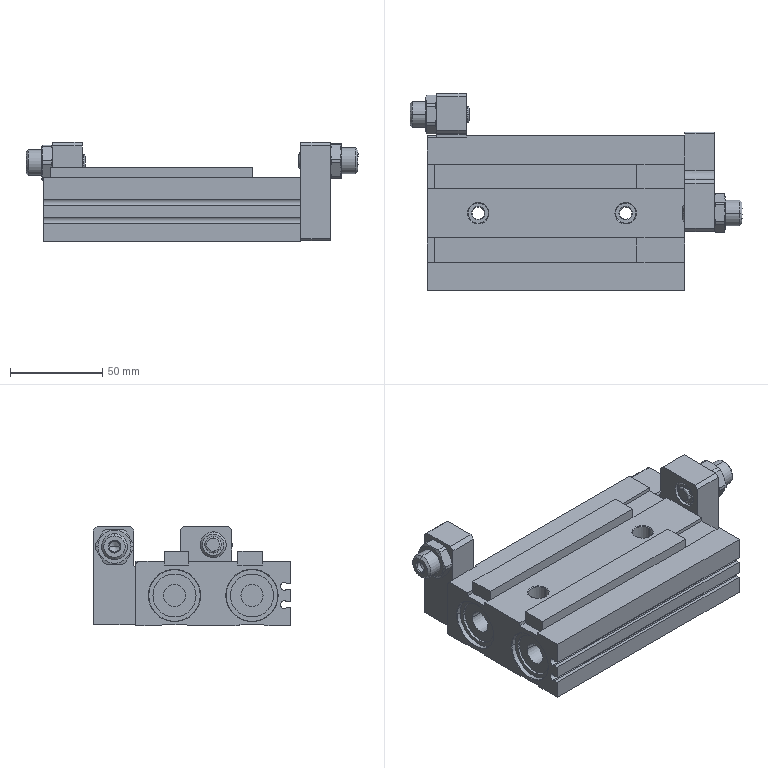Part | SolidWorks | features BaseBody 1 | 1 solid | 370 faces | box 179.95 x 107 x 54.1 mm | volume 360209 mm3 | plane 140 | cylinder 130 | cone 84 | spline 16 | commonest cylinder face diameters 9 x12 21 x12 6 x9 4 x8 4.917 x8 6.647 x8